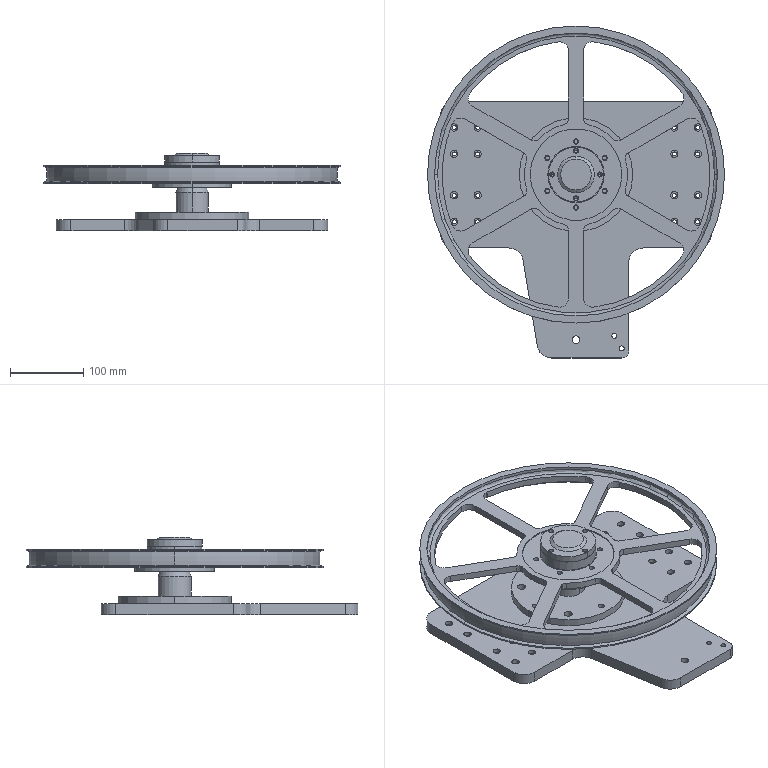Part | SolidWorks | 13 solids | 820 faces | box 405 x 452.5 x 105 mm | volume 2366410 mm3 | cylinder 398 | plane 142 | sphere 132 | torus 100 | cone 48 | commonest cylinder face diameters 0.4 x40 5 x36 5.5 x32 10 x32 1.57 x24 7 x20